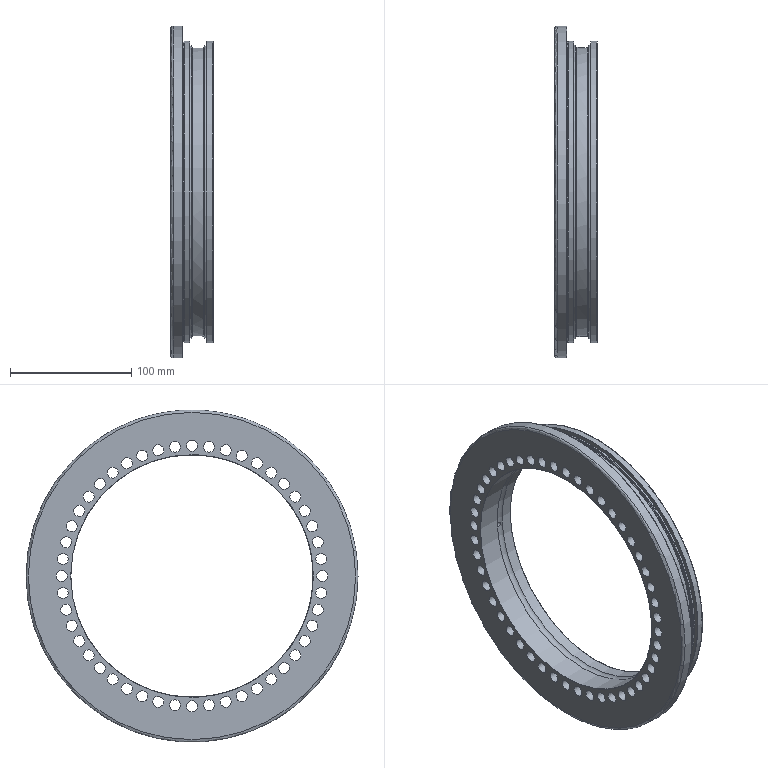Part | STEP file | Part | 1 solid | 83 faces | box 34.993 x 274 x 274 mm | volume 543480 mm3 | cylinder 57 | torus 11 | cone 8 | plane 7 | commonest cylinder face diameters 9 x48 200 x2 242.3 x2 248.6 x2 3.5 x1 238.614 x1